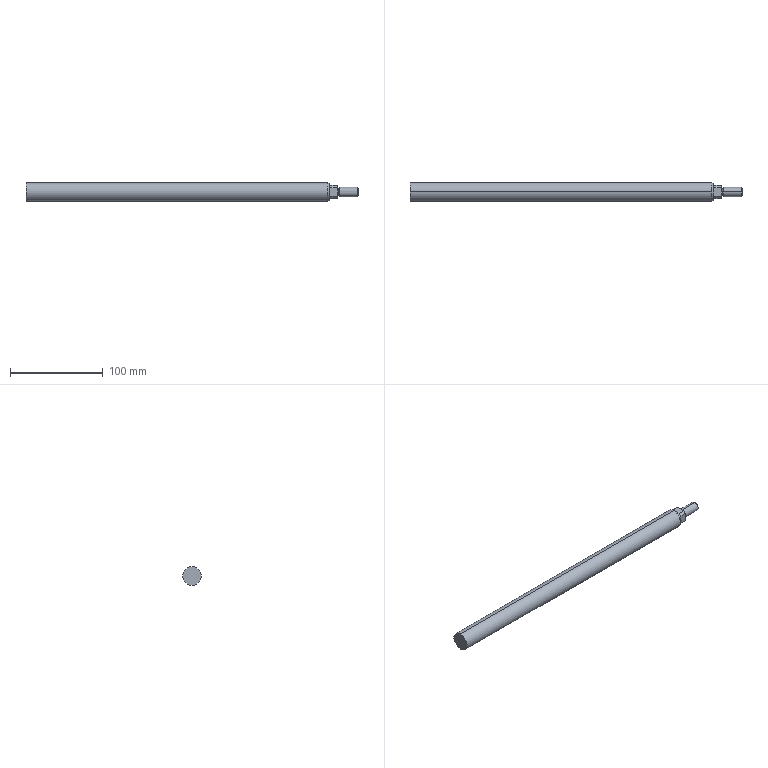Part | STEP file | Guide wheel mechanism revised.sldasm-Part-469 | 1 solid | 28 faces | box 357.5 x 20 x 20 mm | volume 105918 mm3 | plane 14 | cylinder 10 | cone 4 | commonest cylinder face diameters 8 x2 10 x2 17 x2 19 x2 20 x2
STEP:
#1=CARTESIAN_POINT('',(42.5,0.,4.233));
#2=VERTEX_POINT('',#1);
#3=CARTESIAN_POINT('',(42.5,0.,-4.233));
#4=VERTEX_POINT('',#3);
#5=CARTESIAN_POINT('',(42.5,0.,0.));
#6=DIRECTION('',(-1.,0.,0.));
#7=DIRECTION('',(0.,0.,1.));
#8=AXIS2_PLACEMENT_3D('',#5,#6,#7);
#9=CIRCLE('',#8,4.233);
#10=EDGE_CURVE('',#2,#4,#9,.T.);
#11=ORIENTED_EDGE('',*,*,#10,.T.);
#12=CARTESIAN_POINT('',(41.733,0.,-5.));
#13=VERTEX_POINT('',#12);
#14=CARTESIAN_POINT('',(42.5,0.,-4.233));
#15=DIRECTION('',(-0.7071,0.,-0.7071));
#16=VECTOR('',#15,1000.);
#17=LINE('',#14,#16);
#18=EDGE_CURVE('',#4,#13,#17,.T.);
#19=ORIENTED_EDGE('',*,*,#18,.T.);
#20=CARTESIAN_POINT('',(41.733,0.,5.));
#21=VERTEX_POINT('',#20);
#22=CARTESIAN_POINT('',(41.733,0.,0.));
#23=DIRECTION('',(-1.,0.,0.));
#24=DIRECTION('',(0.,0.,1.));
#25=AXIS2_PLACEMENT_3D('',#22,#23,#24);
#26=CIRCLE('',#25,5.);
#27=EDGE_CURVE('',#21,#13,#26,.T.);
#28=ORIENTED_EDGE('',*,*,#27,.F.);
#29=CARTESIAN_POINT('',(42.5,0.,4.233));
#30=DIRECTION('',(-0.7071,0.,0.7071));
#31=VECTOR('',#30,1000.);
#32=LINE('',#29,#31);
#33=EDGE_CURVE('',#2,#21,#32,.T.);
#34=ORIENTED_EDGE('',*,*,#33,.F.);
#35=EDGE_LOOP('',(#11,#19,#28,#34));
#36=FACE_OUTER_BOUND('',#35,.T.);
#37=CARTESIAN_POINT('',(42.5,0.,0.));
#38=DIRECTION('',(-1.,0.,0.));
#39=DIRECTION('',(0.,0.,1.));
#40=AXIS2_PLACEMENT_3D('',#37,#38,#39);
#41=CONICAL_SURFACE('',#40,4.233,0.7854);
#42=ADVANCED_FACE('',(#36),#41,.T.);
#43=ORIENTED_EDGE('',*,*,#27,.T.);
#44=CARTESIAN_POINT('',(22.267,0.,-5.));
#45=VERTEX_POINT('',#44);
#46=CARTESIAN_POINT('',(42.5,0.,-5.));
#47=DIRECTION('',(-1.,0.,0.));
#48=VECTOR('',#47,1000.);
#49=LINE('',#46,#48);
#50=EDGE_CURVE('',#13,#45,#49,.T.);
#51=ORIENTED_EDGE('',*,*,#50,.T.);
#52=CARTESIAN_POINT('',(22.267,0.,5.));
#53=VERTEX_POINT('',#52);
#54=CARTESIAN_POINT('',(22.267,0.,0.));
#55=DIRECTION('',(-1.,0.,0.));
#56=DIRECTION('',(0.,0.,1.));
#57=AXIS2_PLACEMENT_3D('',#54,#55,#56);
#58=CIRCLE('',#57,5.);
#59=EDGE_CURVE('',#53,#45,#58,.T.);
#60=ORIENTED_EDGE('',*,*,#59,.F.);
#61=CARTESIAN_POINT('',(42.5,0.,5.));
#62=DIRECTION('',(-1.,0.,0.));
#63=VECTOR('',#62,1000.);
#64=LINE('',#61,#63);
#65=EDGE_CURVE('',#21,#53,#64,.T.);
#66=ORIENTED_EDGE('',*,*,#65,.F.);
#67=EDGE_LOOP('',(#43,#51,#60,#66));
#68=FACE_OUTER_BOUND('',#67,.T.);
#69=CARTESIAN_POINT('',(42.5,0.,0.));
#70=DIRECTION('',(-1.,0.,0.));
#71=DIRECTION('',(0.,0.,1.));
#72=AXIS2_PLACEMENT_3D('',#69,#70,#71);
#73=CYLINDRICAL_SURFACE('',#72,5.);
#74=ADVANCED_FACE('',(#68),#73,.T.);
#75=CARTESIAN_POINT('',(21.5,0.,4.233));
#76=VERTEX_POINT('',#75);
#77=CARTESIAN_POINT('',(21.5,0.,-4.233));
#78=VERTEX_POINT('',#77);
#79=CARTESIAN_POINT('',(21.5,0.,0.));
#80=DIRECTION('',(-1.,0.,0.));
#81=DIRECTION('',(0.,0.,1.));
#82=AXIS2_PLACEMENT_3D('',#79,#80,#81);
#83=CIRCLE('',#82,4.233);
#84=EDGE_CURVE('',#76,#78,#83,.T.);
#85=ORIENTED_EDGE('',*,*,#84,.F.);
#86=CARTESIAN_POINT('',(22.267,0.,5.));
#87=DIRECTION('',(0.7071,0.,0.7071));
#88=VECTOR('',#87,1000.);
#89=LINE('',#86,#88);
#90=EDGE_CURVE('',#76,#53,#89,.T.);
#91=ORIENTED_EDGE('',*,*,#90,.T.);
#92=ORIENTED_EDGE('',*,*,#59,.T.);
#93=CARTESIAN_POINT('',(22.267,0.,-5.));
#94=DIRECTION('',(0.7071,0.,-0.7071));
#95=VECTOR('',#94,1000.);
#96=LINE('',#93,#95);
#97=EDGE_CURVE('',#78,#45,#96,.T.);
#98=ORIENTED_EDGE('',*,*,#97,.F.);
#99=EDGE_LOOP('',(#85,#91,#92,#98));
#100=FACE_OUTER_BOUND('',#99,.T.);
#101=CARTESIAN_POINT('',(22.267,0.,0.));
#102=DIRECTION('',(1.,0.,0.));
#103=DIRECTION('',(0.,0.,-1.));
#104=AXIS2_PLACEMENT_3D('',#101,#102,#103);
#105=CONICAL_SURFACE('',#104,5.,0.7854);
#106=ADVANCED_FACE('',(#100),#105,.T.);
#107=CARTESIAN_POINT('',(21.5,0.,4.));
#108=VERTEX_POINT('',#107);
#109=CARTESIAN_POINT('',(21.5,0.,-4.));
#110=VERTEX_POINT('',#109);
#111=CARTESIAN_POINT('',(21.5,0.,0.));
#112=DIRECTION('',(-1.,0.,0.));
#113=DIRECTION('',(0.,0.,1.));
#114=AXIS2_PLACEMENT_3D('',#111,#112,#113);
#115=CIRCLE('',#114,4.);
#116=EDGE_CURVE('',#108,#110,#115,.T.);
#117=ORIENTED_EDGE('',*,*,#116,.T.);
#118=CARTESIAN_POINT('',(20.5,0.,-4.));
#119=VERTEX_POINT('',#118);
#120=CARTESIAN_POINT('',(42.5,0.,-4.));
#121=DIRECTION('',(-1.,0.,0.));
#122=VECTOR('',#121,1000.);
#123=LINE('',#120,#122);
#124=EDGE_CURVE('',#110,#119,#123,.T.);
#125=ORIENTED_EDGE('',*,*,#124,.T.);
#126=CARTESIAN_POINT('',(20.5,0.,4.));
#127=VERTEX_POINT('',#126);
#128=CARTESIAN_POINT('',(20.5,0.,0.));
#129=DIRECTION('',(-1.,0.,0.));
#130=DIRECTION('',(0.,0.,1.));
#131=AXIS2_PLACEMENT_3D('',#128,#129,#130);
#132=CIRCLE('',#131,4.);
#133=EDGE_CURVE('',#127,#119,#132,.T.);
#134=ORIENTED_EDGE('',*,*,#133,.F.);
#135=CARTESIAN_POINT('',(42.5,0.,4.));
#136=DIRECTION('',(-1.,0.,0.));
#137=VECTOR('',#136,1000.);
#138=LINE('',#135,#137);
#139=EDGE_CURVE('',#108,#127,#138,.T.);
#140=ORIENTED_EDGE('',*,*,#139,.F.);
#141=EDGE_LOOP('',(#117,#125,#134,#140));
#142=FACE_OUTER_BOUND('',#141,.T.);
#143=CARTESIAN_POINT('',(42.5,0.,0.));
#144=DIRECTION('',(-1.,0.,0.));
#145=DIRECTION('',(0.,0.,1.));
#146=AXIS2_PLACEMENT_3D('',#143,#144,#145);
#147=CYLINDRICAL_SURFACE('',#146,4.);
#148=ADVANCED_FACE('',(#142),#147,.T.);
#149=CARTESIAN_POINT('',(11.5,0.,9.5));
#150=VERTEX_POINT('',#149);
#151=CARTESIAN_POINT('',(11.5,0.,-9.5));
#152=VERTEX_POINT('',#151);
#153=CARTESIAN_POINT('',(11.5,0.,0.));
#154=DIRECTION('',(-1.,0.,0.));
#155=DIRECTION('',(0.,0.,1.));
#156=AXIS2_PLACEMENT_3D('',#153,#154,#155);
#157=CIRCLE('',#156,9.5);
#158=EDGE_CURVE('',#150,#152,#157,.T.);
#159=ORIENTED_EDGE('',*,*,#158,.T.);
#160=CARTESIAN_POINT('',(10.,0.,-9.5));
#161=VERTEX_POINT('',#160);
#162=CARTESIAN_POINT('',(42.5,0.,-9.5));
#163=DIRECTION('',(-1.,0.,0.));
#164=VECTOR('',#163,1000.);
#165=LINE('',#162,#164);
#166=EDGE_CURVE('',#152,#161,#165,.T.);
#167=ORIENTED_EDGE('',*,*,#166,.T.);
#168=CARTESIAN_POINT('',(10.,0.,9.5));
#169=VERTEX_POINT('',#168);
#170=CARTESIAN_POINT('',(10.,0.,0.));
#171=DIRECTION('',(-1.,0.,0.));
#172=DIRECTION('',(0.,0.,1.));
#173=AXIS2_PLACEMENT_3D('',#170,#171,#172);
#174=CIRCLE('',#173,9.5);
#175=EDGE_CURVE('',#169,#161,#174,.T.);
#176=ORIENTED_EDGE('',*,*,#175,.F.);
#177=CARTESIAN_POINT('',(42.5,0.,9.5));
#178=DIRECTION('',(-1.,0.,0.));
#179=VECTOR('',#178,1000.);
#180=LINE('',#177,#179);
#181=EDGE_CURVE('',#150,#169,#180,.T.);
#182=ORIENTED_EDGE('',*,*,#181,.F.);
#183=EDGE_LOOP('',(#159,#167,#176,#182));
#184=FACE_OUTER_BOUND('',#183,.T.);
#185=CARTESIAN_POINT('',(42.5,0.,0.));
#186=DIRECTION('',(-1.,0.,0.));
#187=DIRECTION('',(0.,0.,1.));
#188=AXIS2_PLACEMENT_3D('',#185,#186,#187);
#189=CYLINDRICAL_SURFACE('',#188,9.5);
#190=ADVANCED_FACE('',(#184),#189,.T.);
#191=CARTESIAN_POINT('',(10.,0.,10.));
#192=VERTEX_POINT('',#191);
#193=CARTESIAN_POINT('',(10.,0.,-10.));
#194=VERTEX_POINT('',#193);
#195=CARTESIAN_POINT('',(10.,0.,0.));
#196=DIRECTION('',(-1.,0.,0.));
#197=DIRECTION('',(0.,0.,1.));
#198=AXIS2_PLACEMENT_3D('',#195,#196,#197);
#199=CIRCLE('',#198,10.);
#200=EDGE_CURVE('',#192,#194,#199,.T.);
#201=ORIENTED_EDGE('',*,*,#200,.T.);
#202=CARTESIAN_POINT('',(-315.,0.,-10.));
#203=VERTEX_POINT('',#202);
#204=CARTESIAN_POINT('',(42.5,0.,-10.));
#205=DIRECTION('',(-1.,0.,0.));
#206=VECTOR('',#205,1000.);
#207=LINE('',#204,#206);
#208=EDGE_CURVE('',#194,#203,#207,.T.);
#209=ORIENTED_EDGE('',*,*,#208,.T.);
#210=CARTESIAN_POINT('',(-315.,0.,10.));
#211=VERTEX_POINT('',#210);
#212=CARTESIAN_POINT('',(-315.,0.,0.));
#213=DIRECTION('',(-1.,0.,0.));
#214=DIRECTION('',(0.,0.,1.));
#215=AXIS2_PLACEMENT_3D('',#212,#213,#214);
#216=CIRCLE('',#215,10.);
#217=EDGE_CURVE('',#211,#203,#216,.T.);
#218=ORIENTED_EDGE('',*,*,#217,.F.);
#219=CARTESIAN_POINT('',(42.5,0.,10.));
#220=DIRECTION('',(-1.,0.,0.));
#221=VECTOR('',#220,1000.);
#222=LINE('',#219,#221);
#223=EDGE_CURVE('',#192,#211,#222,.T.);
#224=ORIENTED_EDGE('',*,*,#223,.F.);
#225=EDGE_LOOP('',(#201,#209,#218,#224));
#226=FACE_OUTER_BOUND('',#225,.T.);
#227=CARTESIAN_POINT('',(42.5,0.,0.));
#228=DIRECTION('',(-1.,0.,0.));
#229=DIRECTION('',(0.,0.,1.));
#230=AXIS2_PLACEMENT_3D('',#227,#228,#229);
#231=CYLINDRICAL_SURFACE('',#230,10.);
#232=ADVANCED_FACE('',(#226),#231,.T.);
#233=CARTESIAN_POINT('',(12.,0.,-8.5));
#234=VERTEX_POINT('',#233);
#235=CARTESIAN_POINT('',(12.,4.822,-7.));
#236=VERTEX_POINT('',#235);
#237=CARTESIAN_POINT('',(12.,0.,0.));
#238=DIRECTION('',(1.,0.,0.));
#239=DIRECTION('',(0.,0.,-1.));
#240=AXIS2_PLACEMENT_3D('',#237,#238,#239);
#241=CIRCLE('',#240,8.5);
#242=EDGE_CURVE('',#234,#236,#241,.T.);
#243=ORIENTED_EDGE('',*,*,#242,.F.);
#244=CARTESIAN_POINT('',(11.5,0.,-8.5));
#245=VERTEX_POINT('',#244);
#246=CARTESIAN_POINT('',(42.5,0.,-8.5));
#247=DIRECTION('',(-1.,0.,0.));
#248=VECTOR('',#247,1000.);
#249=LINE('',#246,#248);
#250=EDGE_CURVE('',#234,#245,#249,.T.);
#251=ORIENTED_EDGE('',*,*,#250,.T.);
#252=CARTESIAN_POINT('',(11.5,0.,8.5));
#253=VERTEX_POINT('',#252);
#254=CARTESIAN_POINT('',(11.5,0.,0.));
#255=DIRECTION('',(-1.,0.,0.));
#256=DIRECTION('',(0.,0.,1.));
#257=AXIS2_PLACEMENT_3D('',#254,#255,#256);
#258=CIRCLE('',#257,8.5);
#259=EDGE_CURVE('',#253,#245,#258,.T.);
#260=ORIENTED_EDGE('',*,*,#259,.F.);
#261=CARTESIAN_POINT('',(12.,0.,8.5));
#262=VERTEX_POINT('',#261);
#263=CARTESIAN_POINT('',(42.5,0.,8.5));
#264=DIRECTION('',(-1.,0.,0.));
#265=VECTOR('',#264,1000.);
#266=LINE('',#263,#265);
#267=EDGE_CURVE('',#262,#253,#266,.T.);
#268=ORIENTED_EDGE('',*,*,#267,.F.);
#269=CARTESIAN_POINT('',(12.,4.822,7.));
#270=VERTEX_POINT('',#269);
#271=CARTESIAN_POINT('',(12.,0.,0.));
#272=DIRECTION('',(1.,0.,0.));
#273=DIRECTION('',(0.,0.,-1.));
#274=AXIS2_PLACEMENT_3D('',#271,#272,#273);
#275=CIRCLE('',#274,8.5);
#276=EDGE_CURVE('',#270,#262,#275,.T.);
#277=ORIENTED_EDGE('',*,*,#276,.F.);
#278=CARTESIAN_POINT('',(20.5,4.822,7.));
#279=VERTEX_POINT('',#278);
#280=CARTESIAN_POINT('',(42.5,4.822,7.));
#281=DIRECTION('',(-1.,0.,0.));
#282=VECTOR('',#281,1000.);
#283=LINE('',#280,#282);
#284=EDGE_CURVE('',#279,#270,#283,.T.);
#285=ORIENTED_EDGE('',*,*,#284,.F.);
#286=CARTESIAN_POINT('',(20.5,7.,4.822));
#287=VERTEX_POINT('',#286);
#288=CARTESIAN_POINT('',(20.5,0.,0.));
#289=DIRECTION('',(-1.,0.,0.));
#290=DIRECTION('',(0.,0.,1.));
#291=AXIS2_PLACEMENT_3D('',#288,#289,#290);
#292=CIRCLE('',#291,8.5);
#293=EDGE_CURVE('',#279,#287,#292,.T.);
#294=ORIENTED_EDGE('',*,*,#293,.T.);
#295=CARTESIAN_POINT('',(12.,7.,4.822));
#296=VERTEX_POINT('',#295);
#297=CARTESIAN_POINT('',(42.5,7.,4.822));
#298=DIRECTION('',(1.,0.,0.));
#299=VECTOR('',#298,1000.);
#300=LINE('',#297,#299);
#301=EDGE_CURVE('',#296,#287,#300,.T.);
#302=ORIENTED_EDGE('',*,*,#301,.F.);
#303=CARTESIAN_POINT('',(12.,7.,-4.822));
#304=VERTEX_POINT('',#303);
#305=CARTESIAN_POINT('',(12.,0.,0.));
#306=DIRECTION('',(1.,0.,0.));
#307=DIRECTION('',(0.,0.,-1.));
#308=AXIS2_PLACEMENT_3D('',#305,#306,#307);
#309=CIRCLE('',#308,8.5);
#310=EDGE_CURVE('',#304,#296,#309,.T.);
#311=ORIENTED_EDGE('',*,*,#310,.F.);
#312=CARTESIAN_POINT('',(20.5,7.,-4.822));
#313=VERTEX_POINT('',#312);
#314=CARTESIAN_POINT('',(42.5,7.,-4.822));
#315=DIRECTION('',(-1.,0.,0.));
#316=VECTOR('',#315,1000.);
#317=LINE('',#314,#316);
#318=EDGE_CURVE('',#313,#304,#317,.T.);
#319=ORIENTED_EDGE('',*,*,#318,.F.);
#320=CARTESIAN_POINT('',(20.5,4.822,-7.));
#321=VERTEX_POINT('',#320);
#322=CARTESIAN_POINT('',(20.5,0.,0.));
#323=DIRECTION('',(-1.,0.,0.));
#324=DIRECTION('',(0.,0.,1.));
#325=AXIS2_PLACEMENT_3D('',#322,#323,#324);
#326=CIRCLE('',#325,8.5);
#327=EDGE_CURVE('',#313,#321,#326,.T.);
#328=ORIENTED_EDGE('',*,*,#327,.T.);
#329=CARTESIAN_POINT('',(42.5,4.822,-7.));
#330=DIRECTION('',(1.,0.,0.));
#331=VECTOR('',#330,1000.);
#332=LINE('',#329,#331);
#333=EDGE_CURVE('',#236,#321,#332,.T.);
#334=ORIENTED_EDGE('',*,*,#333,.F.);
#335=EDGE_LOOP('',(#243,#251,#260,#268,#277,#285,#294,#302,#311,#319,#328,#334));
#336=FACE_OUTER_BOUND('',#335,.T.);
#337=CARTESIAN_POINT('',(42.5,0.,0.));
#338=DIRECTION('',(-1.,0.,0.));
#339=DIRECTION('',(0.,0.,1.));
#340=AXIS2_PLACEMENT_3D('',#337,#338,#339);
#341=CYLINDRICAL_SURFACE('',#340,8.5);
#342=ADVANCED_FACE('',(#336),#341,.T.);
#343=ORIENTED_EDGE('',*,*,#250,.F.);
#344=CARTESIAN_POINT('',(12.,-4.822,-7.));
#345=VERTEX_POINT('',#344);
#346=CARTESIAN_POINT('',(12.,0.,0.));
#347=DIRECTION('',(1.,0.,0.));
#348=DIRECTION('',(0.,0.,-1.));
#349=AXIS2_PLACEMENT_3D('',#346,#347,#348);
#350=CIRCLE('',#349,8.5);
#351=EDGE_CURVE('',#345,#234,#350,.T.);
#352=ORIENTED_EDGE('',*,*,#351,.F.);
#353=CARTESIAN_POINT('',(20.5,-4.822,-7.));
#354=VERTEX_POINT('',#353);
#355=CARTESIAN_POINT('',(42.5,-4.822,-7.));
#356=DIRECTION('',(-1.,0.,0.));
#357=VECTOR('',#356,1000.);
#358=LINE('',#355,#357);
#359=EDGE_CURVE('',#354,#345,#358,.T.);
#360=ORIENTED_EDGE('',*,*,#359,.F.);
#361=CARTESIAN_POINT('',(20.5,-7.,-4.822));
#362=VERTEX_POINT('',#361);
#363=CARTESIAN_POINT('',(20.5,0.,0.));
#364=DIRECTION('',(-1.,0.,0.));
#365=DIRECTION('',(0.,0.,1.));
#366=AXIS2_PLACEMENT_3D('',#363,#364,#365);
#367=CIRCLE('',#366,8.5);
#368=EDGE_CURVE('',#354,#362,#367,.T.);
#369=ORIENTED_EDGE('',*,*,#368,.T.);
#370=CARTESIAN_POINT('',(12.,-7.,-4.822));
#371=VERTEX_POINT('',#370);
#372=CARTESIAN_POINT('',(42.5,-7.,-4.822));
#373=DIRECTION('',(1.,0.,0.));
#374=VECTOR('',#373,1000.);
#375=LINE('',#372,#374);
#376=EDGE_CURVE('',#371,#362,#375,.T.);
#377=ORIENTED_EDGE('',*,*,#376,.F.);
#378=CARTESIAN_POINT('',(12.,-7.,4.822));
#379=VERTEX_POINT('',#378);
#380=CARTESIAN_POINT('',(12.,0.,0.));
#381=DIRECTION('',(1.,0.,0.));
#382=DIRECTION('',(0.,0.,-1.));
#383=AXIS2_PLACEMENT_3D('',#380,#381,#382);
#384=CIRCLE('',#383,8.5);
#385=EDGE_CURVE('',#379,#371,#384,.T.);
#386=ORIENTED_EDGE('',*,*,#385,.F.);
#387=CARTESIAN_POINT('',(20.5,-7.,4.822));
#388=VERTEX_POINT('',#387);
#389=CARTESIAN_POINT('',(42.5,-7.,4.822));
#390=DIRECTION('',(-1.,0.,0.));
#391=VECTOR('',#390,1000.);
#392=LINE('',#389,#391);
#393=EDGE_CURVE('',#388,#379,#392,.T.);
#394=ORIENTED_EDGE('',*,*,#393,.F.);
#395=CARTESIAN_POINT('',(20.5,-4.822,7.));
#396=VERTEX_POINT('',#395);
#397=CARTESIAN_POINT('',(20.5,0.,0.));
#398=DIRECTION('',(-1.,0.,0.));
#399=DIRECTION('',(0.,0.,1.));
#400=AXIS2_PLACEMENT_3D('',#397,#398,#399);
#401=CIRCLE('',#400,8.5);
#402=EDGE_CURVE('',#388,#396,#401,.T.);
#403=ORIENTED_EDGE('',*,*,#402,.T.);
#404=CARTESIAN_POINT('',(12.,-4.822,7.));
#405=VERTEX_POINT('',#404);
#406=CARTESIAN_POINT('',(42.5,-4.822,7.));
#407=DIRECTION('',(1.,0.,0.));
#408=VECTOR('',#407,1000.);
#409=LINE('',#406,#408);
#410=EDGE_CURVE('',#405,#396,#409,.T.);
#411=ORIENTED_EDGE('',*,*,#410,.F.);
#412=CARTESIAN_POINT('',(12.,0.,0.));
#413=DIRECTION('',(1.,0.,0.));
#414=DIRECTION('',(0.,0.,-1.));
#415=AXIS2_PLACEMENT_3D('',#412,#413,#414);
#416=CIRCLE('',#415,8.5);
#417=EDGE_CURVE('',#262,#405,#416,.T.);
#418=ORIENTED_EDGE('',*,*,#417,.F.);
#419=ORIENTED_EDGE('',*,*,#267,.T.);
#420=CARTESIAN_POINT('',(11.5,0.,0.));
#421=DIRECTION('',(-1.,0.,0.));
#422=DIRECTION('',(0.,0.,1.));
#423=AXIS2_PLACEMENT_3D('',#420,#421,#422);
#424=CIRCLE('',#423,8.5);
#425=EDGE_CURVE('',#245,#253,#424,.T.);
#426=ORIENTED_EDGE('',*,*,#425,.F.);
#427=EDGE_LOOP('',(#343,#352,#360,#369,#377,#386,#394,#403,#411,#418,#419,#426));
#428=FACE_OUTER_BOUND('',#427,.T.);
#429=CARTESIAN_POINT('',(42.5,0.,0.));
#430=DIRECTION('',(-1.,0.,0.));
#431=DIRECTION('',(0.,0.,1.));
#432=AXIS2_PLACEMENT_3D('',#429,#430,#431);
#433=CYLINDRICAL_SURFACE('',#432,8.5);
#434=ADVANCED_FACE('',(#428),#433,.T.);
#435=ORIENTED_EDGE('',*,*,#133,.T.);
#436=CARTESIAN_POINT('',(20.5,0.,0.));
#437=DIRECTION('',(-1.,0.,0.));
#438=DIRECTION('',(0.,0.,1.));
#439=AXIS2_PLACEMENT_3D('',#436,#437,#438);
#440=CIRCLE('',#439,4.);
#441=EDGE_CURVE('',#119,#127,#440,.T.);
#442=ORIENTED_EDGE('',*,*,#441,.T.);
#443=EDGE_LOOP('',(#435,#442));
#444=FACE_BOUND('',#443,.T.);
#445=CARTESIAN_POINT('',(20.5,7.,0.));
#446=DIRECTION('',(0.,0.,-1.));
#447=VECTOR('',#446,1000.);
#448=LINE('',#445,#447);
#449=EDGE_CURVE('',#287,#313,#448,.T.);
#450=ORIENTED_EDGE('',*,*,#449,.F.);
#451=ORIENTED_EDGE('',*,*,#293,.F.);
#452=CARTESIAN_POINT('',(20.5,8.5,7.));
#453=DIRECTION('',(0.,1.,0.));
#454=VECTOR('',#453,1000.);
#455=LINE('',#452,#454);
#456=EDGE_CURVE('',#396,#279,#455,.T.);
#457=ORIENTED_EDGE('',*,*,#456,.F.);
#458=ORIENTED_EDGE('',*,*,#402,.F.);
#459=CARTESIAN_POINT('',(20.5,-7.,0.));
#460=DIRECTION('',(0.,0.,1.));
#461=VECTOR('',#460,1000.);
#462=LINE('',#459,#461);
#463=EDGE_CURVE('',#362,#388,#462,.T.);
#464=ORIENTED_EDGE('',*,*,#463,.F.);
#465=ORIENTED_EDGE('',*,*,#368,.F.);
#466=CARTESIAN_POINT('',(20.5,8.5,-7.));
#467=DIRECTION('',(0.,-1.,0.));
#468=VECTOR('',#467,1000.);
#469=LINE('',#466,#468);
#470=EDGE_CURVE('',#321,#354,#469,.T.);
#471=ORIENTED_EDGE('',*,*,#470,.F.);
#472=ORIENTED_EDGE('',*,*,#327,.F.);
#473=EDGE_LOOP('',(#450,#451,#457,#458,#464,#465,#471,#472));
#474=FACE_OUTER_BOUND('',#473,.T.);
#475=CARTESIAN_POINT('',(20.5,8.5,0.));
#476=DIRECTION('',(-1.,0.,0.));
#477=DIRECTION('',(0.,0.,1.));
#478=AXIS2_PLACEMENT_3D('',#475,#476,#477);
#479=PLANE('',#478);
#480=ADVANCED_FACE('',(#444,#474),#479,.F.);
#481=ORIENTED_EDGE('',*,*,#217,.T.);
#482=CARTESIAN_POINT('',(-315.,0.,0.));
#483=DIRECTION('',(-1.,0.,0.));
#484=DIRECTION('',(0.,0.,1.));
#485=AXIS2_PLACEMENT_3D('',#482,#483,#484);
#486=CIRCLE('',#485,10.);
#487=EDGE_CURVE('',#203,#211,#486,.T.);
#488=ORIENTED_EDGE('',*,*,#487,.T.);
#489=EDGE_LOOP('',(#481,#488));
#490=FACE_OUTER_BOUND('',#489,.T.);
#491=CARTESIAN_POINT('',(-315.,0.,0.));
#492=DIRECTION('',(1.,0.,0.));
#493=DIRECTION('',(0.,0.,-1.));
#494=AXIS2_PLACEMENT_3D('',#491,#492,#493);
#495=PLANE('',#494);
#496=ADVANCED_FACE('',(#490),#495,.F.);
#497=ORIENTED_EDGE('',*,*,#208,.F.);
#498=CARTESIAN_POINT('',(10.,0.,0.));
#499=DIRECTION('',(-1.,0.,0.));
#500=DIRECTION('',(0.,0.,1.));
#501=AXIS2_PLACEMENT_3D('',#498,#499,#500);
#502=CIRCLE('',#501,10.);
#503=EDGE_CURVE('',#194,#192,#502,.T.);
#504=ORIENTED_EDGE('',*,*,#503,.T.);
#505=ORIENTED_EDGE('',*,*,#223,.T.);
#506=ORIENTED_EDGE('',*,*,#487,.F.);
#507=EDGE_LOOP('',(#497,#504,#505,#506));
#508=FACE_OUTER_BOUND('',#507,.T.);
#509=CARTESIAN_POINT('',(42.5,0.,0.));
#510=DIRECTION('',(-1.,0.,0.));
#511=DIRECTION('',(0.,0.,1.));
#512=AXIS2_PLACEMENT_3D('',#509,#510,#511);
#513=CYLINDRICAL_SURFACE('',#512,10.);
#514=ADVANCED_FACE('',(#508),#513,.T.);
#515=ORIENTED_EDGE('',*,*,#200,.F.);
#516=ORIENTED_EDGE('',*,*,#503,.F.);
#517=EDGE_LOOP('',(#515,#516));
#518=FACE_OUTER_BOUND('',#517,.T.);
#519=ORIENTED_EDGE('',*,*,#175,.T.);
#520=CARTESIAN_POINT('',(10.,0.,0.));
#521=DIRECTION('',(-1.,0.,0.));
#522=DIRECTION('',(0.,0.,1.));
#523=AXIS2_PLACEMENT_3D('',#520,#521,#522);
#524=CIRCLE('',#523,9.5);
#525=EDGE_CURVE('',#161,#169,#524,.T.);
#526=ORIENTED_EDGE('',*,*,#525,.T.);
#527=EDGE_LOOP('',(#519,#526));
#528=FACE_BOUND('',#527,.T.);
#529=CARTESIAN_POINT('',(10.,10.,0.));
#530=DIRECTION('',(-1.,0.,0.));
#531=DIRECTION('',(0.,0.,1.));
#532=AXIS2_PLACEMENT_3D('',#529,#530,#531);
#533=PLANE('',#532);
#534=ADVANCED_FACE('',(#518,#528),#533,.F.);
#535=ORIENTED_EDGE('',*,*,#166,.F.);
#536=CARTESIAN_POINT('',(11.5,0.,0.));
#537=DIRECTION('',(-1.,0.,0.));
#538=DIRECTION('',(0.,0.,1.));
#539=AXIS2_PLACEMENT_3D('',#536,#537,#538);
#540=CIRCLE('',#539,9.5);
#541=EDGE_CURVE('',#152,#150,#540,.T.);
#542=ORIENTED_EDGE('',*,*,#541,.T.);
#543=ORIENTED_EDGE('',*,*,#181,.T.);
#544=ORIENTED_EDGE('',*,*,#525,.F.);
#545=EDGE_LOOP('',(#535,#542,#543,#544));
#546=FACE_OUTER_BOUND('',#545,.T.);
#547=CARTESIAN_POINT('',(42.5,0.,0.));
#548=DIRECTION('',(-1.,0.,0.));
#549=DIRECTION('',(0.,0.,1.));
#550=AXIS2_PLACEMENT_3D('',#547,#548,#549);
#551=CYLINDRICAL_SURFACE('',#550,9.5);
#552=ADVANCED_FACE('',(#546),#551,.T.);
#553=ORIENTED_EDGE('',*,*,#158,.F.);
#554=ORIENTED_EDGE('',*,*,#541,.F.);
#555=EDGE_LOOP('',(#553,#554));
#556=FACE_OUTER_BOUND('',#555,.T.);
#557=ORIENTED_EDGE('',*,*,#259,.T.);
#558=ORIENTED_EDGE('',*,*,#425,.T.);
#559=EDGE_LOOP('',(#557,#558));
#560=FACE_BOUND('',#559,.T.);
#561=CARTESIAN_POINT('',(11.5,9.5,0.));
#562=DIRECTION('',(-1.,0.,0.));
#563=DIRECTION('',(0.,0.,1.));
#564=AXIS2_PLACEMENT_3D('',#561,#562,#563);
#565=PLANE('',#564);
#566=ADVANCED_FACE('',(#556,#560),#565,.F.);
#567=ORIENTED_EDGE('',*,*,#124,.F.);
#568=CARTESIAN_POINT('',(21.5,0.,0.));
#569=DIRECTION('',(-1.,0.,0.));
#570=DIRECTION('',(0.,0.,1.));
#571=AXIS2_PLACEMENT_3D('',#568,#569,#570);
#572=CIRCLE('',#571,4.);
#573=EDGE_CURVE('',#110,#108,#572,.T.);
#574=ORIENTED_EDGE('',*,*,#573,.T.);
#575=ORIENTED_EDGE('',*,*,#139,.T.);
#576=ORIENTED_EDGE('',*,*,#441,.F.);
#577=EDGE_LOOP('',(#567,#574,#575,#576));
#578=FACE_OUTER_BOUND('',#577,.T.);
#579=CARTESIAN_POINT('',(42.5,0.,0.));
#580=DIRECTION('',(-1.,0.,0.));
#581=DIRECTION('',(0.,0.,1.));
#582=AXIS2_PLACEMENT_3D('',#579,#580,#581);
#583=CYLINDRICAL_SURFACE('',#582,4.);
#584=ADVANCED_FACE('',(#578),#583,.T.);
#585=ORIENTED_EDGE('',*,*,#116,.F.);
#586=ORIENTED_EDGE('',*,*,#573,.F.);
#587=EDGE_LOOP('',(#585,#586));
#588=FACE_BOUND('',#587,.T.);
#589=CARTESIAN_POINT('',(21.5,0.,0.));
#590=DIRECTION('',(-1.,0.,0.));
#591=DIRECTION('',(0.,0.,1.));
#592=AXIS2_PLACEMENT_3D('',#589,#590,#591);
#593=CIRCLE('',#592,4.233);
#594=EDGE_CURVE('',#78,#76,#593,.T.);
#595=ORIENTED_EDGE('',*,*,#594,.T.);
#596=ORIENTED_EDGE('',*,*,#84,.T.);
#597=EDGE_LOOP('',(#595,#596));
#598=FACE_OUTER_BOUND('',#597,.T.);
#599=CARTESIAN_POINT('',(21.5,4.,0.));
#600=DIRECTION('',(1.,0.,0.));
#601=DIRECTION('',(0.,0.,-1.));
#602=AXIS2_PLACEMENT_3D('',#599,#600,#601);
#603=PLANE('',#602);
#604=ADVANCED_FACE('',(#588,#598),#603,.F.);
#605=ORIENTED_EDGE('',*,*,#90,.F.);
#606=ORIENTED_EDGE('',*,*,#594,.F.);
#607=ORIENTED_EDGE('',*,*,#97,.T.);
#608=CARTESIAN_POINT('',(22.267,0.,0.));
#609=DIRECTION('',(-1.,0.,0.));
#610=DIRECTION('',(0.,0.,1.));
#611=AXIS2_PLACEMENT_3D('',#608,#609,#610);
#612=CIRCLE('',#611,5.);
#613=EDGE_CURVE('',#45,#53,#612,.T.);
#614=ORIENTED_EDGE('',*,*,#613,.T.);
#615=EDGE_LOOP('',(#605,#606,#607,#614));
#616=FACE_OUTER_BOUND('',#615,.T.);
#617=CARTESIAN_POINT('',(22.267,0.,0.));
#618=DIRECTION('',(1.,0.,0.));
#619=DIRECTION('',(0.,0.,-1.));
#620=AXIS2_PLACEMENT_3D('',#617,#618,#619);
#621=CONICAL_SURFACE('',#620,5.,0.7854);
#622=ADVANCED_FACE('',(#616),#621,.T.);
#623=ORIENTED_EDGE('',*,*,#50,.F.);
#624=CARTESIAN_POINT('',(41.733,0.,0.));
#625=DIRECTION('',(-1.,0.,0.));
#626=DIRECTION('',(0.,0.,1.));
#627=AXIS2_PLACEMENT_3D('',#624,#625,#626);
#628=CIRCLE('',#627,5.);
#629=EDGE_CURVE('',#13,#21,#628,.T.);
#630=ORIENTED_EDGE('',*,*,#629,.T.);
#631=ORIENTED_EDGE('',*,*,#65,.T.);
#632=ORIENTED_EDGE('',*,*,#613,.F.);
#633=EDGE_LOOP('',(#623,#630,#631,#632));
#634=FACE_OUTER_BOUND('',#633,.T.);
#635=CARTESIAN_POINT('',(42.5,0.,0.));
#636=DIRECTION('',(-1.,0.,0.));
#637=DIRECTION('',(0.,0.,1.));
#638=AXIS2_PLACEMENT_3D('',#635,#636,#637);
#639=CYLINDRICAL_SURFACE('',#638,5.);
#640=ADVANCED_FACE('',(#634),#639,.T.);
#641=ORIENTED_EDGE('',*,*,#18,.F.);
#642=CARTESIAN_POINT('',(42.5,0.,0.));
#643=DIRECTION('',(-1.,0.,0.));
#644=DIRECTION('',(0.,0.,1.));
#645=AXIS2_PLACEMENT_3D('',#642,#643,#644);
#646=CIRCLE('',#645,4.233);
#647=EDGE_CURVE('',#4,#2,#646,.T.);
#648=ORIENTED_EDGE('',*,*,#647,.T.);
#649=ORIENTED_EDGE('',*,*,#33,.T.);
#650=ORIENTED_EDGE('',*,*,#629,.F.);
#651=EDGE_LOOP('',(#641,#648,#649,#650));
#652=FACE_OUTER_BOUND('',#651,.T.);
#653=CARTESIAN_POINT('',(42.5,0.,0.));
#654=DIRECTION('',(-1.,0.,0.));
#655=DIRECTION('',(0.,0.,1.));
#656=AXIS2_PLACEMENT_3D('',#653,#654,#655);
#657=CONICAL_SURFACE('',#656,4.233,0.7854);
#658=ADVANCED_FACE('',(#652),#657,.T.);
#659=ORIENTED_EDGE('',*,*,#10,.F.);
#660=ORIENTED_EDGE('',*,*,#647,.F.);
#661=EDGE_LOOP('',(#659,#660));
#662=FACE_OUTER_BOUND('',#661,.T.);
#663=CARTESIAN_POINT('',(42.5,4.233,0.));
#664=DIRECTION('',(-1.,0.,0.));
#665=DIRECTION('',(0.,0.,1.));
#666=AXIS2_PLACEMENT_3D('',#663,#664,#665);
#667=PLANE('',#666);
#668=ADVANCED_FACE('',(#662),#667,.F.);
#669=ORIENTED_EDGE('',*,*,#284,.T.);
#670=CARTESIAN_POINT('',(12.,7.,7.));
#671=DIRECTION('',(0.,-1.,0.));
#672=VECTOR('',#671,1000.);
#673=LINE('',#670,#672);
#674=EDGE_CURVE('',#270,#405,#673,.T.);
#675=ORIENTED_EDGE('',*,*,#674,.T.);
#676=ORIENTED_EDGE('',*,*,#410,.T.);
#677=ORIENTED_EDGE('',*,*,#456,.T.);
#678=EDGE_LOOP('',(#669,#675,#676,#677));
#679=FACE_OUTER_BOUND('',#678,.T.);
#680=CARTESIAN_POINT('',(12.,7.,7.));
#681=DIRECTION('',(0.,0.,1.));
#682=DIRECTION('',(1.,0.,0.));
#683=AXIS2_PLACEMENT_3D('',#680,#681,#682);
#684=PLANE('',#683);
#685=ADVANCED_FACE('',(#679),#684,.T.);
#686=ORIENTED_EDGE('',*,*,#276,.T.);
#687=ORIENTED_EDGE('',*,*,#417,.T.);
#688=ORIENTED_EDGE('',*,*,#674,.F.);
#689=EDGE_LOOP('',(#686,#687,#688));
#690=FACE_OUTER_BOUND('',#689,.T.);
#691=CARTESIAN_POINT('',(12.,0.,0.));
#692=DIRECTION('',(1.,0.,0.));
#693=DIRECTION('',(0.,0.,-1.));
#694=AXIS2_PLACEMENT_3D('',#691,#692,#693);
#695=PLANE('',#694);
#696=ADVANCED_FACE('',(#690),#695,.T.);
#697=ORIENTED_EDGE('',*,*,#393,.T.);
#698=CARTESIAN_POINT('',(12.,-7.,7.));
#699=DIRECTION('',(0.,0.,-1.));
#700=VECTOR('',#699,1000.);
#701=LINE('',#698,#700);
#702=EDGE_CURVE('',#379,#371,#701,.T.);
#703=ORIENTED_EDGE('',*,*,#702,.T.);
#704=ORIENTED_EDGE('',*,*,#376,.T.);
#705=ORIENTED_EDGE('',*,*,#463,.T.);
#706=EDGE_LOOP('',(#697,#703,#704,#705));
#707=FACE_OUTER_BOUND('',#706,.T.);
#708=CARTESIAN_POINT('',(12.,-7.,7.));
#709=DIRECTION('',(0.,-1.,0.));
#710=DIRECTION('',(0.,0.,-1.));
#711=AXIS2_PLACEMENT_3D('',#708,#709,#710);
#712=PLANE('',#711);
#713=ADVANCED_FACE('',(#707),#712,.T.);
#714=ORIENTED_EDGE('',*,*,#385,.T.);
#715=ORIENTED_EDGE('',*,*,#702,.F.);
#716=EDGE_LOOP('',(#714,#715));
#717=FACE_OUTER_BOUND('',#716,.T.);
#718=CARTESIAN_POINT('',(12.,0.,0.));
#719=DIRECTION('',(1.,0.,0.));
#720=DIRECTION('',(0.,0.,-1.));
#721=AXIS2_PLACEMENT_3D('',#718,#719,#720);
#722=PLANE('',#721);
#723=ADVANCED_FACE('',(#717),#722,.T.);
#724=ORIENTED_EDGE('',*,*,#359,.T.);
#725=CARTESIAN_POINT('',(12.,-7.,-7.));
#726=DIRECTION('',(0.,1.,0.));
#727=VECTOR('',#726,1000.);
#728=LINE('',#725,#727);
#729=EDGE_CURVE('',#345,#236,#728,.T.);
#730=ORIENTED_EDGE('',*,*,#729,.T.);
#731=ORIENTED_EDGE('',*,*,#333,.T.);
#732=ORIENTED_EDGE('',*,*,#470,.T.);
#733=EDGE_LOOP('',(#724,#730,#731,#732));
#734=FACE_OUTER_BOUND('',#733,.T.);
#735=CARTESIAN_POINT('',(12.,-7.,-7.));
#736=DIRECTION('',(0.,0.,-1.));
#737=DIRECTION('',(-1.,0.,0.));
#738=AXIS2_PLACEMENT_3D('',#735,#736,#737);
#739=PLANE('',#738);
#740=ADVANCED_FACE('',(#734),#739,.T.);
#741=ORIENTED_EDGE('',*,*,#351,.T.);
#742=ORIENTED_EDGE('',*,*,#242,.T.);
#743=ORIENTED_EDGE('',*,*,#729,.F.);
#744=EDGE_LOOP('',(#741,#742,#743));
#745=FACE_OUTER_BOUND('',#744,.T.);
#746=CARTESIAN_POINT('',(12.,0.,0.));
#747=DIRECTION('',(1.,0.,0.));
#748=DIRECTION('',(0.,0.,-1.));
#749=AXIS2_PLACEMENT_3D('',#746,#747,#748);
#750=PLANE('',#749);
#751=ADVANCED_FACE('',(#745),#750,.T.);
#752=ORIENTED_EDGE('',*,*,#310,.T.);
#753=CARTESIAN_POINT('',(12.,7.,-7.));
#754=DIRECTION('',(0.,0.,1.));
#755=VECTOR('',#754,1000.);
#756=LINE('',#753,#755);
#757=EDGE_CURVE('',#304,#296,#756,.T.);
#758=ORIENTED_EDGE('',*,*,#757,.F.);
#759=EDGE_LOOP('',(#752,#758));
#760=FACE_OUTER_BOUND('',#759,.T.);
#761=CARTESIAN_POINT('',(12.,0.,0.));
#762=DIRECTION('',(1.,0.,0.));
#763=DIRECTION('',(0.,0.,-1.));
#764=AXIS2_PLACEMENT_3D('',#761,#762,#763);
#765=PLANE('',#764);
#766=ADVANCED_FACE('',(#760),#765,.T.);
#767=ORIENTED_EDGE('',*,*,#318,.T.);
#768=ORIENTED_EDGE('',*,*,#757,.T.);
#769=ORIENTED_EDGE('',*,*,#301,.T.);
#770=ORIENTED_EDGE('',*,*,#449,.T.);
#771=EDGE_LOOP('',(#767,#768,#769,#770));
#772=FACE_OUTER_BOUND('',#771,.T.);
#773=CARTESIAN_POINT('',(12.,7.,-7.));
#774=DIRECTION('',(0.,1.,0.));
#775=DIRECTION('',(0.,0.,1.));
#776=AXIS2_PLACEMENT_3D('',#773,#774,#775);
#777=PLANE('',#776);
#778=ADVANCED_FACE('',(#772),#777,.T.);
#779=CLOSED_SHELL('',(#42,#74,#106,#148,#190,#232,#342,#434,#480,#496,#514,#534,#552,#566,#584,#604,#622,#640,#658,#668,#685,#696,#713,#723,#740,#751,#766,#778));
#780=MANIFOLD_SOLID_BREP('',#779);
#781=CARTESIAN_POINT('',(0.,0.,0.));
#782=DIRECTION('',(0.,0.,1.));
#783=DIRECTION('',(1.,0.,0.));
#784=AXIS2_PLACEMENT_3D('',#781,#782,#783);
#785=(LENGTH_UNIT()NAMED_UNIT(*)SI_UNIT(.MILLI.,.METRE.));
#786=UNCERTAINTY_MEASURE_WITH_UNIT(LENGTH_MEASURE(0.00001),#785,'','');
#787=(NAMED_UNIT(*)PLANE_ANGLE_UNIT()SI_UNIT($,.RADIAN.));
#788=(NAMED_UNIT(*)SI_UNIT($,.STERADIAN.)SOLID_ANGLE_UNIT());
#789=(GEOMETRIC_REPRESENTATION_CONTEXT(3)GLOBAL_UNCERTAINTY_ASSIGNED_CONTEXT((#786))GLOBAL_UNIT_ASSIGNED_CONTEXT((#785,#787,#788))REPRESENTATION_CONTEXT('',''));
#790=ADVANCED_BREP_SHAPE_REPRESENTATION('',(#780,#784),#789);